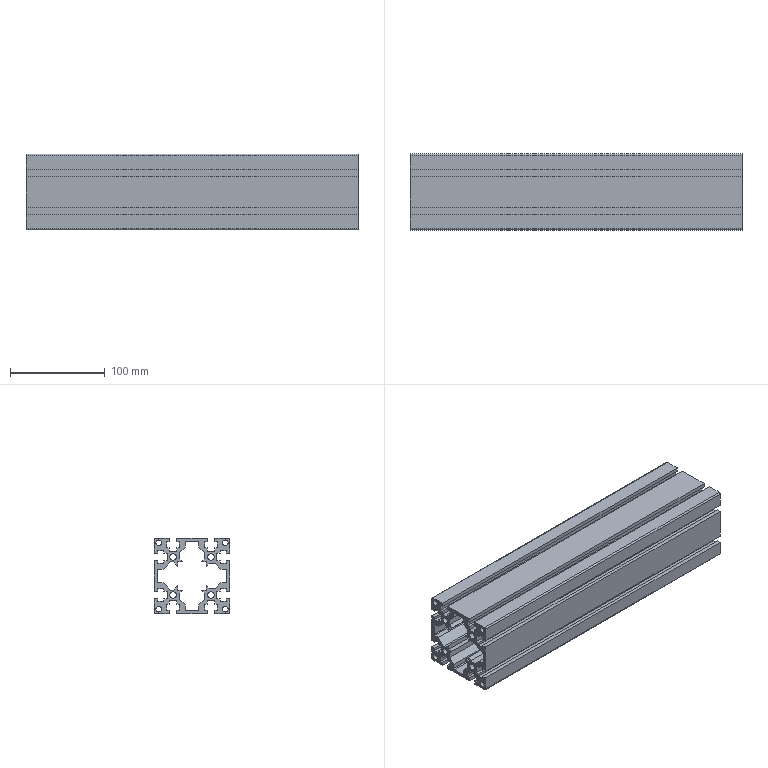Part | SolidWorks | features ICE 1, WeldMemberFeat 1, WeldmentFeature 1 | 1 solid | 174 faces | box 350 x 80 x 80 mm | volume 801157 mm3 | plane 146 | cylinder 28 | commonest cylinder face diameters 2 x8 6 x8 6.8 x8 3 x4